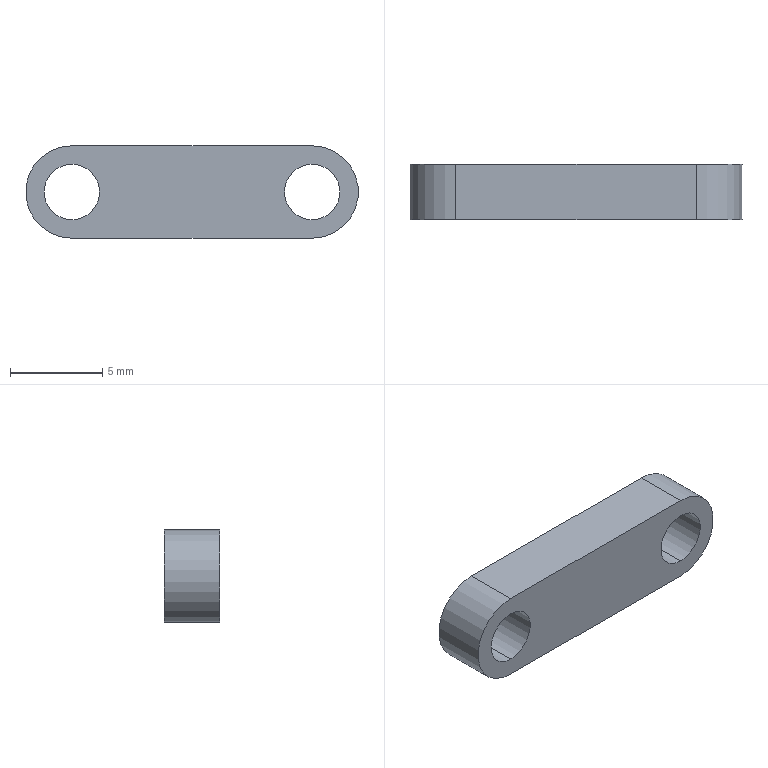Part | SolidWorks | features Extrusion 1 | 1 solid | 10 faces | box 18 x 3 x 5 mm | volume 211.493 mm3 | cylinder 6 | plane 4 | commonest cylinder face diameters 3 x4 5 x2
STEP:
#1=CARTESIAN_POINT('',(13.,3.,-1.5));
#2=VERTEX_POINT('',#1);
#3=CARTESIAN_POINT('',(13.,3.,1.5));
#4=VERTEX_POINT('',#3);
#5=CARTESIAN_POINT('',(13.,3.,0.));
#6=DIRECTION('',(0.,1.,0.));
#7=DIRECTION('',(0.,0.,1.));
#8=AXIS2_PLACEMENT_3D('',#5,#6,#7);
#9=CIRCLE('',#8,1.5);
#10=EDGE_CURVE('',#2,#4,#9,.T.);
#11=ORIENTED_EDGE('',*,*,#10,.T.);
#12=CARTESIAN_POINT('',(13.,0.,1.5));
#13=VERTEX_POINT('',#12);
#14=CARTESIAN_POINT('',(13.,3.,1.5));
#15=DIRECTION('',(0.,-1.,0.));
#16=VECTOR('',#15,1000.);
#17=LINE('',#14,#16);
#18=EDGE_CURVE('',#4,#13,#17,.T.);
#19=ORIENTED_EDGE('',*,*,#18,.T.);
#20=CARTESIAN_POINT('',(13.,0.,-1.5));
#21=VERTEX_POINT('',#20);
#22=CARTESIAN_POINT('',(13.,0.,0.));
#23=DIRECTION('',(0.,1.,0.));
#24=DIRECTION('',(0.,0.,1.));
#25=AXIS2_PLACEMENT_3D('',#22,#23,#24);
#26=CIRCLE('',#25,1.5);
#27=EDGE_CURVE('',#21,#13,#26,.T.);
#28=ORIENTED_EDGE('',*,*,#27,.F.);
#29=CARTESIAN_POINT('',(13.,3.,-1.5));
#30=DIRECTION('',(0.,-1.,0.));
#31=VECTOR('',#30,1000.);
#32=LINE('',#29,#31);
#33=EDGE_CURVE('',#2,#21,#32,.T.);
#34=ORIENTED_EDGE('',*,*,#33,.F.);
#35=EDGE_LOOP('',(#11,#19,#28,#34));
#36=FACE_OUTER_BOUND('',#35,.T.);
#37=CARTESIAN_POINT('',(13.,3.,0.));
#38=DIRECTION('',(0.,-1.,0.));
#39=DIRECTION('',(0.,0.,-1.));
#40=AXIS2_PLACEMENT_3D('',#37,#38,#39);
#41=CYLINDRICAL_SURFACE('',#40,1.5);
#42=ADVANCED_FACE('',(#36),#41,.F.);
#43=CARTESIAN_POINT('',(0.,3.,-1.5));
#44=VERTEX_POINT('',#43);
#45=CARTESIAN_POINT('',(0.,3.,1.5));
#46=VERTEX_POINT('',#45);
#47=CARTESIAN_POINT('',(0.,3.,0.));
#48=DIRECTION('',(0.,1.,0.));
#49=DIRECTION('',(0.,0.,1.));
#50=AXIS2_PLACEMENT_3D('',#47,#48,#49);
#51=CIRCLE('',#50,1.5);
#52=EDGE_CURVE('',#44,#46,#51,.T.);
#53=ORIENTED_EDGE('',*,*,#52,.T.);
#54=CARTESIAN_POINT('',(0.,0.,1.5));
#55=VERTEX_POINT('',#54);
#56=CARTESIAN_POINT('',(0.,3.,1.5));
#57=DIRECTION('',(0.,-1.,0.));
#58=VECTOR('',#57,1000.);
#59=LINE('',#56,#58);
#60=EDGE_CURVE('',#46,#55,#59,.T.);
#61=ORIENTED_EDGE('',*,*,#60,.T.);
#62=CARTESIAN_POINT('',(0.,0.,-1.5));
#63=VERTEX_POINT('',#62);
#64=CARTESIAN_POINT('',(0.,0.,0.));
#65=DIRECTION('',(0.,1.,0.));
#66=DIRECTION('',(0.,0.,1.));
#67=AXIS2_PLACEMENT_3D('',#64,#65,#66);
#68=CIRCLE('',#67,1.5);
#69=EDGE_CURVE('',#63,#55,#68,.T.);
#70=ORIENTED_EDGE('',*,*,#69,.F.);
#71=CARTESIAN_POINT('',(0.,3.,-1.5));
#72=DIRECTION('',(0.,-1.,0.));
#73=VECTOR('',#72,1000.);
#74=LINE('',#71,#73);
#75=EDGE_CURVE('',#44,#63,#74,.T.);
#76=ORIENTED_EDGE('',*,*,#75,.F.);
#77=EDGE_LOOP('',(#53,#61,#70,#76));
#78=FACE_OUTER_BOUND('',#77,.T.);
#79=CARTESIAN_POINT('',(0.,3.,0.));
#80=DIRECTION('',(0.,-1.,0.));
#81=DIRECTION('',(0.,0.,-1.));
#82=AXIS2_PLACEMENT_3D('',#79,#80,#81);
#83=CYLINDRICAL_SURFACE('',#82,1.5);
#84=ADVANCED_FACE('',(#78),#83,.F.);
#85=ORIENTED_EDGE('',*,*,#52,.F.);
#86=CARTESIAN_POINT('',(0.,3.,0.));
#87=DIRECTION('',(0.,1.,0.));
#88=DIRECTION('',(0.,0.,1.));
#89=AXIS2_PLACEMENT_3D('',#86,#87,#88);
#90=CIRCLE('',#89,1.5);
#91=EDGE_CURVE('',#46,#44,#90,.T.);
#92=ORIENTED_EDGE('',*,*,#91,.F.);
#93=EDGE_LOOP('',(#85,#92));
#94=FACE_BOUND('',#93,.T.);
#95=CARTESIAN_POINT('',(0.,3.,-2.5));
#96=VERTEX_POINT('',#95);
#97=CARTESIAN_POINT('',(0.,3.,2.5));
#98=VERTEX_POINT('',#97);
#99=CARTESIAN_POINT('',(0.,3.,0.));
#100=DIRECTION('',(0.,1.,0.));
#101=DIRECTION('',(0.,0.,1.));
#102=AXIS2_PLACEMENT_3D('',#99,#100,#101);
#103=CIRCLE('',#102,2.5);
#104=EDGE_CURVE('',#96,#98,#103,.T.);
#105=ORIENTED_EDGE('',*,*,#104,.T.);
#106=CARTESIAN_POINT('',(13.,3.,2.5));
#107=VERTEX_POINT('',#106);
#108=CARTESIAN_POINT('',(0.,3.,2.5));
#109=DIRECTION('',(1.,0.,0.));
#110=VECTOR('',#109,1000.);
#111=LINE('',#108,#110);
#112=EDGE_CURVE('',#98,#107,#111,.T.);
#113=ORIENTED_EDGE('',*,*,#112,.T.);
#114=CARTESIAN_POINT('',(13.,3.,-2.5));
#115=VERTEX_POINT('',#114);
#116=CARTESIAN_POINT('',(13.,3.,0.));
#117=DIRECTION('',(0.,1.,0.));
#118=DIRECTION('',(0.,0.,1.));
#119=AXIS2_PLACEMENT_3D('',#116,#117,#118);
#120=CIRCLE('',#119,2.5);
#121=EDGE_CURVE('',#107,#115,#120,.T.);
#122=ORIENTED_EDGE('',*,*,#121,.T.);
#123=CARTESIAN_POINT('',(0.,3.,-2.5));
#124=DIRECTION('',(-1.,0.,0.));
#125=VECTOR('',#124,1000.);
#126=LINE('',#123,#125);
#127=EDGE_CURVE('',#115,#96,#126,.T.);
#128=ORIENTED_EDGE('',*,*,#127,.T.);
#129=EDGE_LOOP('',(#105,#113,#122,#128));
#130=FACE_OUTER_BOUND('',#129,.T.);
#131=ORIENTED_EDGE('',*,*,#10,.F.);
#132=CARTESIAN_POINT('',(13.,3.,0.));
#133=DIRECTION('',(0.,1.,0.));
#134=DIRECTION('',(0.,0.,1.));
#135=AXIS2_PLACEMENT_3D('',#132,#133,#134);
#136=CIRCLE('',#135,1.5);
#137=EDGE_CURVE('',#4,#2,#136,.T.);
#138=ORIENTED_EDGE('',*,*,#137,.F.);
#139=EDGE_LOOP('',(#131,#138));
#140=FACE_BOUND('',#139,.T.);
#141=CARTESIAN_POINT('',(0.,3.,0.));
#142=DIRECTION('',(0.,1.,0.));
#143=DIRECTION('',(0.,0.,1.));
#144=AXIS2_PLACEMENT_3D('',#141,#142,#143);
#145=PLANE('',#144);
#146=ADVANCED_FACE('',(#94,#130,#140),#145,.T.);
#147=CARTESIAN_POINT('',(0.,0.,-2.5));
#148=VERTEX_POINT('',#147);
#149=CARTESIAN_POINT('',(0.,0.,2.5));
#150=VERTEX_POINT('',#149);
#151=CARTESIAN_POINT('',(0.,0.,0.));
#152=DIRECTION('',(0.,1.,0.));
#153=DIRECTION('',(0.,0.,1.));
#154=AXIS2_PLACEMENT_3D('',#151,#152,#153);
#155=CIRCLE('',#154,2.5);
#156=EDGE_CURVE('',#148,#150,#155,.T.);
#157=ORIENTED_EDGE('',*,*,#156,.F.);
#158=CARTESIAN_POINT('',(13.,0.,-2.5));
#159=VERTEX_POINT('',#158);
#160=CARTESIAN_POINT('',(0.,0.,-2.5));
#161=DIRECTION('',(-1.,0.,0.));
#162=VECTOR('',#161,1000.);
#163=LINE('',#160,#162);
#164=EDGE_CURVE('',#159,#148,#163,.T.);
#165=ORIENTED_EDGE('',*,*,#164,.F.);
#166=CARTESIAN_POINT('',(13.,0.,2.5));
#167=VERTEX_POINT('',#166);
#168=CARTESIAN_POINT('',(13.,0.,0.));
#169=DIRECTION('',(0.,1.,0.));
#170=DIRECTION('',(0.,0.,1.));
#171=AXIS2_PLACEMENT_3D('',#168,#169,#170);
#172=CIRCLE('',#171,2.5);
#173=EDGE_CURVE('',#167,#159,#172,.T.);
#174=ORIENTED_EDGE('',*,*,#173,.F.);
#175=CARTESIAN_POINT('',(0.,0.,2.5));
#176=DIRECTION('',(1.,0.,0.));
#177=VECTOR('',#176,1000.);
#178=LINE('',#175,#177);
#179=EDGE_CURVE('',#150,#167,#178,.T.);
#180=ORIENTED_EDGE('',*,*,#179,.F.);
#181=EDGE_LOOP('',(#157,#165,#174,#180));
#182=FACE_OUTER_BOUND('',#181,.T.);
#183=ORIENTED_EDGE('',*,*,#69,.T.);
#184=CARTESIAN_POINT('',(0.,0.,0.));
#185=DIRECTION('',(0.,1.,0.));
#186=DIRECTION('',(0.,0.,1.));
#187=AXIS2_PLACEMENT_3D('',#184,#185,#186);
#188=CIRCLE('',#187,1.5);
#189=EDGE_CURVE('',#55,#63,#188,.T.);
#190=ORIENTED_EDGE('',*,*,#189,.T.);
#191=EDGE_LOOP('',(#183,#190));
#192=FACE_BOUND('',#191,.T.);
#193=ORIENTED_EDGE('',*,*,#27,.T.);
#194=CARTESIAN_POINT('',(13.,0.,0.));
#195=DIRECTION('',(0.,1.,0.));
#196=DIRECTION('',(0.,0.,1.));
#197=AXIS2_PLACEMENT_3D('',#194,#195,#196);
#198=CIRCLE('',#197,1.5);
#199=EDGE_CURVE('',#13,#21,#198,.T.);
#200=ORIENTED_EDGE('',*,*,#199,.T.);
#201=EDGE_LOOP('',(#193,#200));
#202=FACE_BOUND('',#201,.T.);
#203=CARTESIAN_POINT('',(0.,0.,0.));
#204=DIRECTION('',(0.,1.,0.));
#205=DIRECTION('',(0.,0.,1.));
#206=AXIS2_PLACEMENT_3D('',#203,#204,#205);
#207=PLANE('',#206);
#208=ADVANCED_FACE('',(#182,#192,#202),#207,.F.);
#209=ORIENTED_EDGE('',*,*,#156,.T.);
#210=CARTESIAN_POINT('',(0.,3.,2.5));
#211=DIRECTION('',(0.,-1.,0.));
#212=VECTOR('',#211,1000.);
#213=LINE('',#210,#212);
#214=EDGE_CURVE('',#98,#150,#213,.T.);
#215=ORIENTED_EDGE('',*,*,#214,.F.);
#216=ORIENTED_EDGE('',*,*,#104,.F.);
#217=CARTESIAN_POINT('',(0.,3.,-2.5));
#218=DIRECTION('',(0.,-1.,0.));
#219=VECTOR('',#218,1000.);
#220=LINE('',#217,#219);
#221=EDGE_CURVE('',#96,#148,#220,.T.);
#222=ORIENTED_EDGE('',*,*,#221,.T.);
#223=EDGE_LOOP('',(#209,#215,#216,#222));
#224=FACE_OUTER_BOUND('',#223,.T.);
#225=CARTESIAN_POINT('',(0.,3.,0.));
#226=DIRECTION('',(0.,-1.,0.));
#227=DIRECTION('',(0.,0.,-1.));
#228=AXIS2_PLACEMENT_3D('',#225,#226,#227);
#229=CYLINDRICAL_SURFACE('',#228,2.5);
#230=ADVANCED_FACE('',(#224),#229,.T.);
#231=ORIENTED_EDGE('',*,*,#179,.T.);
#232=CARTESIAN_POINT('',(13.,3.,2.5));
#233=DIRECTION('',(0.,-1.,0.));
#234=VECTOR('',#233,1000.);
#235=LINE('',#232,#234);
#236=EDGE_CURVE('',#107,#167,#235,.T.);
#237=ORIENTED_EDGE('',*,*,#236,.F.);
#238=ORIENTED_EDGE('',*,*,#112,.F.);
#239=ORIENTED_EDGE('',*,*,#214,.T.);
#240=EDGE_LOOP('',(#231,#237,#238,#239));
#241=FACE_OUTER_BOUND('',#240,.T.);
#242=CARTESIAN_POINT('',(0.,3.,2.5));
#243=DIRECTION('',(0.,0.,-1.));
#244=DIRECTION('',(-1.,0.,0.));
#245=AXIS2_PLACEMENT_3D('',#242,#243,#244);
#246=PLANE('',#245);
#247=ADVANCED_FACE('',(#241),#246,.F.);
#248=ORIENTED_EDGE('',*,*,#173,.T.);
#249=CARTESIAN_POINT('',(13.,3.,-2.5));
#250=DIRECTION('',(0.,-1.,0.));
#251=VECTOR('',#250,1000.);
#252=LINE('',#249,#251);
#253=EDGE_CURVE('',#115,#159,#252,.T.);
#254=ORIENTED_EDGE('',*,*,#253,.F.);
#255=ORIENTED_EDGE('',*,*,#121,.F.);
#256=ORIENTED_EDGE('',*,*,#236,.T.);
#257=EDGE_LOOP('',(#248,#254,#255,#256));
#258=FACE_OUTER_BOUND('',#257,.T.);
#259=CARTESIAN_POINT('',(13.,3.,0.));
#260=DIRECTION('',(0.,-1.,0.));
#261=DIRECTION('',(0.,0.,-1.));
#262=AXIS2_PLACEMENT_3D('',#259,#260,#261);
#263=CYLINDRICAL_SURFACE('',#262,2.5);
#264=ADVANCED_FACE('',(#258),#263,.T.);
#265=ORIENTED_EDGE('',*,*,#164,.T.);
#266=ORIENTED_EDGE('',*,*,#221,.F.);
#267=ORIENTED_EDGE('',*,*,#127,.F.);
#268=ORIENTED_EDGE('',*,*,#253,.T.);
#269=EDGE_LOOP('',(#265,#266,#267,#268));
#270=FACE_OUTER_BOUND('',#269,.T.);
#271=CARTESIAN_POINT('',(0.,3.,-2.5));
#272=DIRECTION('',(0.,0.,1.));
#273=DIRECTION('',(1.,0.,0.));
#274=AXIS2_PLACEMENT_3D('',#271,#272,#273);
#275=PLANE('',#274);
#276=ADVANCED_FACE('',(#270),#275,.F.);
#277=ORIENTED_EDGE('',*,*,#60,.F.);
#278=ORIENTED_EDGE('',*,*,#91,.T.);
#279=ORIENTED_EDGE('',*,*,#75,.T.);
#280=ORIENTED_EDGE('',*,*,#189,.F.);
#281=EDGE_LOOP('',(#277,#278,#279,#280));
#282=FACE_OUTER_BOUND('',#281,.T.);
#283=CARTESIAN_POINT('',(0.,3.,0.));
#284=DIRECTION('',(0.,-1.,0.));
#285=DIRECTION('',(0.,0.,-1.));
#286=AXIS2_PLACEMENT_3D('',#283,#284,#285);
#287=CYLINDRICAL_SURFACE('',#286,1.5);
#288=ADVANCED_FACE('',(#282),#287,.F.);
#289=ORIENTED_EDGE('',*,*,#18,.F.);
#290=ORIENTED_EDGE('',*,*,#137,.T.);
#291=ORIENTED_EDGE('',*,*,#33,.T.);
#292=ORIENTED_EDGE('',*,*,#199,.F.);
#293=EDGE_LOOP('',(#289,#290,#291,#292));
#294=FACE_OUTER_BOUND('',#293,.T.);
#295=CARTESIAN_POINT('',(13.,3.,0.));
#296=DIRECTION('',(0.,-1.,0.));
#297=DIRECTION('',(0.,0.,-1.));
#298=AXIS2_PLACEMENT_3D('',#295,#296,#297);
#299=CYLINDRICAL_SURFACE('',#298,1.5);
#300=ADVANCED_FACE('',(#294),#299,.F.);
#301=CLOSED_SHELL('',(#42,#84,#146,#208,#230,#247,#264,#276,#288,#300));
#302=MANIFOLD_SOLID_BREP('',#301);
#303=CARTESIAN_POINT('',(0.,0.,0.));
#304=DIRECTION('',(0.,0.,1.));
#305=DIRECTION('',(1.,0.,0.));
#306=AXIS2_PLACEMENT_3D('',#303,#304,#305);
#307=(LENGTH_UNIT()NAMED_UNIT(*)SI_UNIT(.MILLI.,.METRE.));
#308=UNCERTAINTY_MEASURE_WITH_UNIT(LENGTH_MEASURE(0.00001),#307,'','');
#309=(NAMED_UNIT(*)PLANE_ANGLE_UNIT()SI_UNIT($,.RADIAN.));
#310=(NAMED_UNIT(*)SI_UNIT($,.STERADIAN.)SOLID_ANGLE_UNIT());
#311=(GEOMETRIC_REPRESENTATION_CONTEXT(3)GLOBAL_UNCERTAINTY_ASSIGNED_CONTEXT((#308))GLOBAL_UNIT_ASSIGNED_CONTEXT((#307,#309,#310))REPRESENTATION_CONTEXT('',''));
#312=ADVANCED_BREP_SHAPE_REPRESENTATION('',(#302,#306),#311);